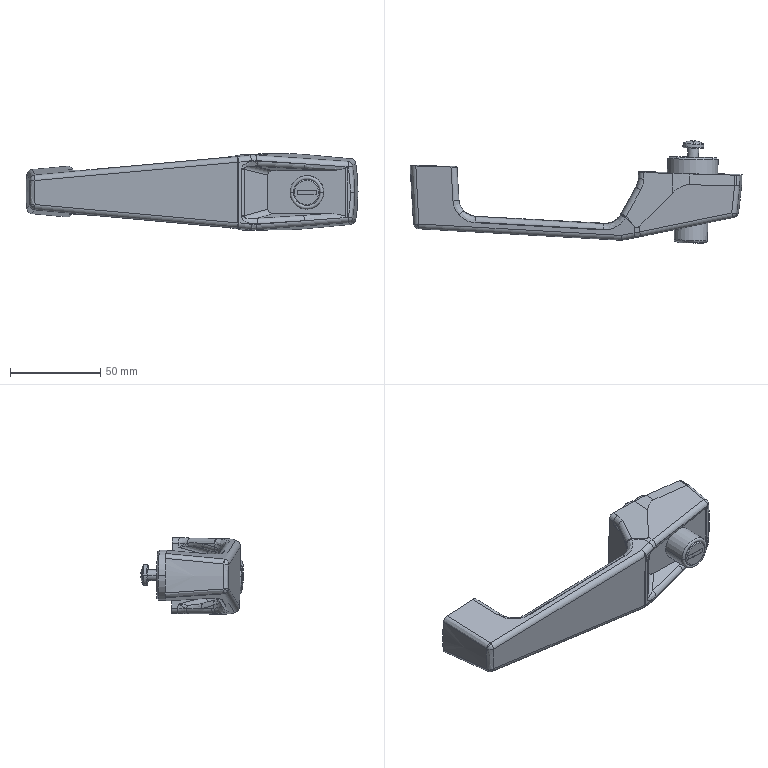Part | NX | features BREP 1 | 1 solid | 208 faces | box 184.421 x 56.842 x 42.453 mm | volume 116707 mm3 | cylinder 75 | plane 42 | spline 31 | cone 23 | torus 20 | sphere 17 | commonest cylinder face diameters 6 x39 0.4 x8 5 x6 20 x6 5.972 x2 6.022 x2